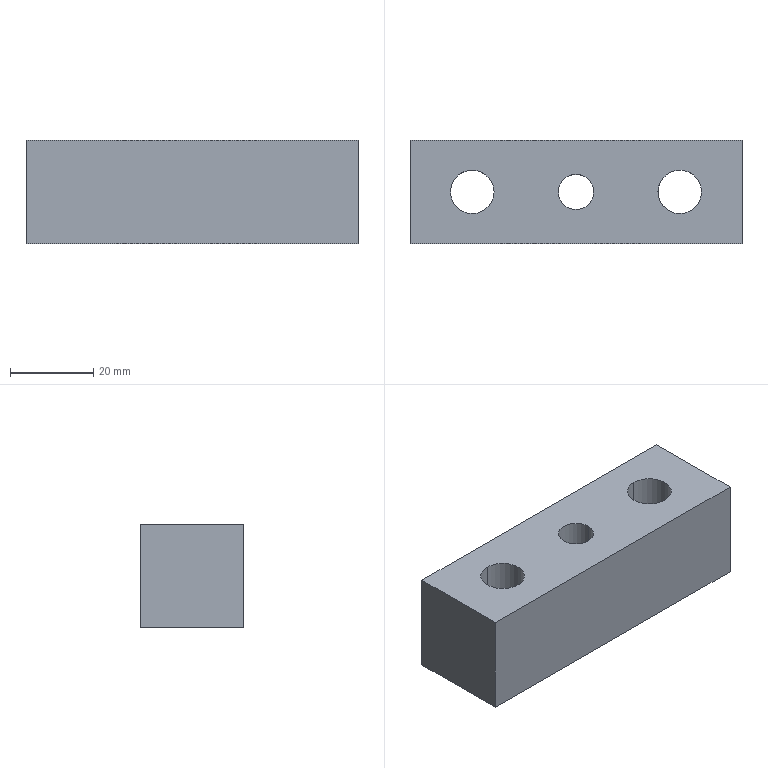Part | STEP file | 1_id1602_x_t | 1 solid | 18 faces | box 80 x 25 x 25 mm | volume 40040 mm3 | cylinder 10 | plane 8 | commonest cylinder face diameters 10.5 x4 17 x4 8.5 x2
STEP:
#1=CARTESIAN_POINT('',(0.,0.,0.));
#2=DIRECTION('',(0.,0.,1.));
#3=DIRECTION('',(1.,0.,0.));
#4=AXIS2_PLACEMENT_3D('',#1,#2,#3);
#5=CARTESIAN_POINT('',(605.45,-32.376,-77.49));
#6=VERTEX_POINT('',#5);
#7=CARTESIAN_POINT('',(613.95,-32.376,-77.49));
#8=VERTEX_POINT('',#7);
#9=CARTESIAN_POINT('',(609.7,-32.376,-77.49));
#10=DIRECTION('',(0.,0.,-1.));
#11=DIRECTION('',(-1.,0.,0.));
#12=AXIS2_PLACEMENT_3D('',#9,#10,#11);
#13=CIRCLE('',#12,4.25);
#14=CARTESIAN_POINT('',(609.7,-32.376,-73.24));
#15=DIRECTION('',(0.,0.,1.));
#16=DIRECTION('',(-1.,0.,0.));
#17=AXIS2_PLACEMENT_3D('',#14,#15,#16);
#18=CYLINDRICAL_SURFACE('',#17,4.25);
#19=CARTESIAN_POINT('',(6.283,-4.25));
#20=DIRECTION('',(-1.,0.));
#21=VECTOR('',#20,1.);
#22=LINE('',#19,#21);
#23=(GEOMETRIC_REPRESENTATION_CONTEXT(2)PARAMETRIC_REPRESENTATION_CONTEXT()REPRESENTATION_CONTEXT('',''));
#24=DEFINITIONAL_REPRESENTATION('',(#22),#23);
#25=PCURVE('',#18,#24);
#26=CARTESIAN_POINT('',(649.7,-44.876,-77.49));
#27=DIRECTION('',(0.,0.,-1.));
#28=DIRECTION('',(1.,0.,0.));
#29=AXIS2_PLACEMENT_3D('',#26,#27,#28);
#30=PLANE('',#29);
#31=CARTESIAN_POINT('',(-40.,-12.5));
#32=DIRECTION('',(-1.,0.));
#33=AXIS2_PLACEMENT_2D('',#31,#32);
#34=CIRCLE('',#33,4.25);
#35=(GEOMETRIC_REPRESENTATION_CONTEXT(2)PARAMETRIC_REPRESENTATION_CONTEXT()REPRESENTATION_CONTEXT('',''));
#36=DEFINITIONAL_REPRESENTATION('',(#34),#35);
#37=PCURVE('',#30,#36);
#38=SURFACE_CURVE('',#13,(#25,#37),.PCURVE_S1.);
#39=EDGE_CURVE('',#6,#8,#38,.T.);
#40=ORIENTED_EDGE('',*,*,#39,.T.);
#41=CARTESIAN_POINT('',(613.95,-32.376,-102.49));
#42=VERTEX_POINT('',#41);
#43=CARTESIAN_POINT('',(613.95,-32.376,-102.49));
#44=DIRECTION('',(0.,0.,1.));
#45=VECTOR('',#44,1.);
#46=LINE('',#43,#45);
#47=CARTESIAN_POINT('',(3.142,-29.25));
#48=DIRECTION('',(0.,1.));
#49=VECTOR('',#48,1.);
#50=LINE('',#47,#49);
#51=(GEOMETRIC_REPRESENTATION_CONTEXT(2)PARAMETRIC_REPRESENTATION_CONTEXT()REPRESENTATION_CONTEXT('',''));
#52=DEFINITIONAL_REPRESENTATION('',(#50),#51);
#53=PCURVE('',#18,#52);
#54=CARTESIAN_POINT('',(609.7,-32.376,-73.24));
#55=DIRECTION('',(0.,0.,1.));
#56=DIRECTION('',(-1.,0.,0.));
#57=AXIS2_PLACEMENT_3D('',#54,#55,#56);
#58=CYLINDRICAL_SURFACE('',#57,4.25);
#59=CARTESIAN_POINT('',(3.142,-29.25));
#60=DIRECTION('',(0.,1.));
#61=VECTOR('',#60,1.);
#62=LINE('',#59,#61);
#63=(GEOMETRIC_REPRESENTATION_CONTEXT(2)PARAMETRIC_REPRESENTATION_CONTEXT()REPRESENTATION_CONTEXT('',''));
#64=DEFINITIONAL_REPRESENTATION('',(#62),#63);
#65=PCURVE('',#58,#64);
#66=SURFACE_CURVE('',#46,(#53,#65),.PCURVE_S1.);
#67=EDGE_CURVE('',#42,#8,#66,.T.);
#68=ORIENTED_EDGE('',*,*,#67,.F.);
#69=CARTESIAN_POINT('',(605.45,-32.376,-102.49));
#70=VERTEX_POINT('',#69);
#71=CARTESIAN_POINT('',(609.7,-32.376,-102.49));
#72=DIRECTION('',(0.,0.,1.));
#73=DIRECTION('',(1.,0.,0.));
#74=AXIS2_PLACEMENT_3D('',#71,#72,#73);
#75=CIRCLE('',#74,4.25);
#76=CARTESIAN_POINT('',(3.142,-29.25));
#77=DIRECTION('',(1.,0.));
#78=VECTOR('',#77,1.);
#79=LINE('',#76,#78);
#80=(GEOMETRIC_REPRESENTATION_CONTEXT(2)PARAMETRIC_REPRESENTATION_CONTEXT()REPRESENTATION_CONTEXT('',''));
#81=DEFINITIONAL_REPRESENTATION('',(#79),#80);
#82=PCURVE('',#18,#81);
#83=CARTESIAN_POINT('',(649.7,-44.876,-102.49));
#84=DIRECTION('',(0.,0.,-1.));
#85=DIRECTION('',(1.,0.,0.));
#86=AXIS2_PLACEMENT_3D('',#83,#84,#85);
#87=PLANE('',#86);
#88=CARTESIAN_POINT('',(-35.75,-12.5));
#89=CARTESIAN_POINT('',(-35.75,-19.861));
#90=CARTESIAN_POINT('',(-42.125,-16.181));
#91=CARTESIAN_POINT('',(-48.5,-12.5));
#92=CARTESIAN_POINT('',(-42.125,-8.819));
#93=CARTESIAN_POINT('',(-35.75,-5.139));
#94=CARTESIAN_POINT('',(-35.75,-12.5));
#95=(BOUNDED_CURVE()B_SPLINE_CURVE(2,(#88,#89,#90,#91,#92,#93,#94),.UNSPECIFIED.,.T.,.F.)B_SPLINE_CURVE_WITH_KNOTS((1,2,2,2,2,1),(-2.094,0.,2.094,4.189,6.283,8.378),.UNSPECIFIED.)CURVE()GEOMETRIC_REPRESENTATION_ITEM()RATIONAL_B_SPLINE_CURVE((1.,0.5,1.,0.5,1.,0.5,1.))REPRESENTATION_ITEM(''));
#96=(GEOMETRIC_REPRESENTATION_CONTEXT(2)PARAMETRIC_REPRESENTATION_CONTEXT()REPRESENTATION_CONTEXT('',''));
#97=DEFINITIONAL_REPRESENTATION('',(#95),#96);
#98=PCURVE('',#87,#97);
#99=SURFACE_CURVE('',#75,(#82,#98),.PCURVE_S1.);
#100=EDGE_CURVE('',#42,#70,#99,.T.);
#101=ORIENTED_EDGE('',*,*,#100,.T.);
#102=CARTESIAN_POINT('',(605.45,-32.376,-102.49));
#103=DIRECTION('',(0.,0.,-1.));
#104=VECTOR('',#103,1.);
#105=LINE('',#102,#104);
#106=CARTESIAN_POINT('',(6.283,-29.25));
#107=DIRECTION('',(0.,-1.));
#108=VECTOR('',#107,1.);
#109=LINE('',#106,#108);
#110=(GEOMETRIC_REPRESENTATION_CONTEXT(2)PARAMETRIC_REPRESENTATION_CONTEXT()REPRESENTATION_CONTEXT('',''));
#111=DEFINITIONAL_REPRESENTATION('',(#109),#110);
#112=PCURVE('',#18,#111);
#113=CARTESIAN_POINT('',(0.,-29.25));
#114=DIRECTION('',(0.,-1.));
#115=VECTOR('',#114,1.);
#116=LINE('',#113,#115);
#117=(GEOMETRIC_REPRESENTATION_CONTEXT(2)PARAMETRIC_REPRESENTATION_CONTEXT()REPRESENTATION_CONTEXT('',''));
#118=DEFINITIONAL_REPRESENTATION('',(#116),#117);
#119=PCURVE('',#58,#118);
#120=SURFACE_CURVE('',#105,(#112,#119),.PCURVE_S1.);
#121=EDGE_CURVE('',#6,#70,#120,.T.);
#122=ORIENTED_EDGE('',*,*,#121,.F.);
#123=EDGE_LOOP('',(#40,#68,#101,#122));
#124=FACE_BOUND('',#123,.F.);
#125=ADVANCED_FACE('',(#124),#18,.F.);
#126=CARTESIAN_POINT('',(649.7,-19.876,-77.49));
#127=VERTEX_POINT('',#126);
#128=CARTESIAN_POINT('',(569.7,-19.876,-77.49));
#129=VERTEX_POINT('',#128);
#130=CARTESIAN_POINT('',(649.7,-19.876,-77.49));
#131=DIRECTION('',(-1.,0.,0.));
#132=VECTOR('',#131,1.);
#133=LINE('',#130,#132);
#134=CARTESIAN_POINT('',(0.,-25.));
#135=DIRECTION('',(-1.,0.));
#136=VECTOR('',#135,1.);
#137=LINE('',#134,#136);
#138=(GEOMETRIC_REPRESENTATION_CONTEXT(2)PARAMETRIC_REPRESENTATION_CONTEXT()REPRESENTATION_CONTEXT('',''));
#139=DEFINITIONAL_REPRESENTATION('',(#137),#138);
#140=PCURVE('',#30,#139);
#141=CARTESIAN_POINT('',(569.7,-19.876,-77.49));
#142=DIRECTION('',(0.,1.,0.));
#143=DIRECTION('',(1.,0.,0.));
#144=AXIS2_PLACEMENT_3D('',#141,#142,#143);
#145=PLANE('',#144);
#146=CARTESIAN_POINT('',(80.,0.));
#147=DIRECTION('',(-1.,0.));
#148=VECTOR('',#147,1.);
#149=LINE('',#146,#148);
#150=(GEOMETRIC_REPRESENTATION_CONTEXT(2)PARAMETRIC_REPRESENTATION_CONTEXT()REPRESENTATION_CONTEXT('',''));
#151=DEFINITIONAL_REPRESENTATION('',(#149),#150);
#152=PCURVE('',#145,#151);
#153=SURFACE_CURVE('',#133,(#140,#152),.PCURVE_S1.);
#154=EDGE_CURVE('',#127,#129,#153,.T.);
#155=ORIENTED_EDGE('',*,*,#154,.T.);
#156=CARTESIAN_POINT('',(569.7,-44.876,-77.49));
#157=VERTEX_POINT('',#156);
#158=CARTESIAN_POINT('',(569.7,-19.876,-77.49));
#159=DIRECTION('',(0.,-1.,0.));
#160=VECTOR('',#159,1.);
#161=LINE('',#158,#160);
#162=CARTESIAN_POINT('',(-80.,-25.));
#163=DIRECTION('',(0.,1.));
#164=VECTOR('',#163,1.);
#165=LINE('',#162,#164);
#166=(GEOMETRIC_REPRESENTATION_CONTEXT(2)PARAMETRIC_REPRESENTATION_CONTEXT()REPRESENTATION_CONTEXT('',''));
#167=DEFINITIONAL_REPRESENTATION('',(#165),#166);
#168=PCURVE('',#30,#167);
#169=CARTESIAN_POINT('',(569.7,-44.876,-77.49));
#170=DIRECTION('',(-1.,0.,0.));
#171=DIRECTION('',(0.,-1.,0.));
#172=AXIS2_PLACEMENT_3D('',#169,#170,#171);
#173=PLANE('',#172);
#174=CARTESIAN_POINT('',(-25.,0.));
#175=DIRECTION('',(1.,0.));
#176=VECTOR('',#175,1.);
#177=LINE('',#174,#176);
#178=(GEOMETRIC_REPRESENTATION_CONTEXT(2)PARAMETRIC_REPRESENTATION_CONTEXT()REPRESENTATION_CONTEXT('',''));
#179=DEFINITIONAL_REPRESENTATION('',(#177),#178);
#180=PCURVE('',#173,#179);
#181=SURFACE_CURVE('',#161,(#168,#180),.PCURVE_S1.);
#182=EDGE_CURVE('',#129,#157,#181,.T.);
#183=ORIENTED_EDGE('',*,*,#182,.T.);
#184=CARTESIAN_POINT('',(649.7,-44.876,-77.49));
#185=VERTEX_POINT('',#184);
#186=CARTESIAN_POINT('',(569.7,-44.876,-77.49));
#187=DIRECTION('',(1.,0.,0.));
#188=VECTOR('',#187,1.);
#189=LINE('',#186,#188);
#190=CARTESIAN_POINT('',(-80.,0.));
#191=DIRECTION('',(1.,0.));
#192=VECTOR('',#191,1.);
#193=LINE('',#190,#192);
#194=(GEOMETRIC_REPRESENTATION_CONTEXT(2)PARAMETRIC_REPRESENTATION_CONTEXT()REPRESENTATION_CONTEXT('',''));
#195=DEFINITIONAL_REPRESENTATION('',(#193),#194);
#196=PCURVE('',#30,#195);
#197=CARTESIAN_POINT('',(649.7,-44.876,-77.49));
#198=DIRECTION('',(0.,-1.,0.));
#199=DIRECTION('',(0.,0.,-1.));
#200=AXIS2_PLACEMENT_3D('',#197,#198,#199);
#201=PLANE('',#200);
#202=CARTESIAN_POINT('',(0.,-80.));
#203=DIRECTION('',(0.,1.));
#204=VECTOR('',#203,1.);
#205=LINE('',#202,#204);
#206=(GEOMETRIC_REPRESENTATION_CONTEXT(2)PARAMETRIC_REPRESENTATION_CONTEXT()REPRESENTATION_CONTEXT('',''));
#207=DEFINITIONAL_REPRESENTATION('',(#205),#206);
#208=PCURVE('',#201,#207);
#209=SURFACE_CURVE('',#189,(#196,#208),.PCURVE_S1.);
#210=EDGE_CURVE('',#157,#185,#209,.T.);
#211=ORIENTED_EDGE('',*,*,#210,.T.);
#212=CARTESIAN_POINT('',(649.7,-44.876,-77.49));
#213=DIRECTION('',(0.,1.,0.));
#214=VECTOR('',#213,1.);
#215=LINE('',#212,#214);
#216=CARTESIAN_POINT('',(0.,0.));
#217=DIRECTION('',(0.,-1.));
#218=VECTOR('',#217,1.);
#219=LINE('',#216,#218);
#220=(GEOMETRIC_REPRESENTATION_CONTEXT(2)PARAMETRIC_REPRESENTATION_CONTEXT()REPRESENTATION_CONTEXT('',''));
#221=DEFINITIONAL_REPRESENTATION('',(#219),#220);
#222=PCURVE('',#30,#221);
#223=CARTESIAN_POINT('',(649.7,-19.876,-77.49));
#224=DIRECTION('',(1.,0.,0.));
#225=DIRECTION('',(0.,0.,1.));
#226=AXIS2_PLACEMENT_3D('',#223,#224,#225);
#227=PLANE('',#226);
#228=CARTESIAN_POINT('',(0.,25.));
#229=DIRECTION('',(0.,-1.));
#230=VECTOR('',#229,1.);
#231=LINE('',#228,#230);
#232=(GEOMETRIC_REPRESENTATION_CONTEXT(2)PARAMETRIC_REPRESENTATION_CONTEXT()REPRESENTATION_CONTEXT('',''));
#233=DEFINITIONAL_REPRESENTATION('',(#231),#232);
#234=PCURVE('',#227,#233);
#235=SURFACE_CURVE('',#215,(#222,#234),.PCURVE_S1.);
#236=EDGE_CURVE('',#185,#127,#235,.T.);
#237=ORIENTED_EDGE('',*,*,#236,.T.);
#238=EDGE_LOOP('',(#155,#183,#211,#237));
#239=FACE_BOUND('',#238,.T.);
#240=CARTESIAN_POINT('',(634.7,-27.126,-77.49));
#241=VERTEX_POINT('',#240);
#242=CARTESIAN_POINT('',(639.95,-32.376,-77.49));
#243=VERTEX_POINT('',#242);
#244=CARTESIAN_POINT('',(634.7,-32.376,-77.49));
#245=DIRECTION('',(0.,0.,-1.));
#246=DIRECTION('',(0.,1.,0.));
#247=AXIS2_PLACEMENT_3D('',#244,#245,#246);
#248=CIRCLE('',#247,5.25);
#249=CARTESIAN_POINT('',(-15.,-12.5));
#250=DIRECTION('',(0.,-1.));
#251=AXIS2_PLACEMENT_2D('',#249,#250);
#252=CIRCLE('',#251,5.25);
#253=(GEOMETRIC_REPRESENTATION_CONTEXT(2)PARAMETRIC_REPRESENTATION_CONTEXT()REPRESENTATION_CONTEXT('',''));
#254=DEFINITIONAL_REPRESENTATION('',(#252),#253);
#255=PCURVE('',#30,#254);
#256=CARTESIAN_POINT('',(634.7,-32.376,-77.24));
#257=DIRECTION('',(0.,0.,1.));
#258=DIRECTION('',(0.,-1.,0.));
#259=AXIS2_PLACEMENT_3D('',#256,#257,#258);
#260=CYLINDRICAL_SURFACE('',#259,5.25);
#261=CARTESIAN_POINT('',(3.142,-0.25));
#262=DIRECTION('',(-1.,0.));
#263=VECTOR('',#262,1.);
#264=LINE('',#261,#263);
#265=(GEOMETRIC_REPRESENTATION_CONTEXT(2)PARAMETRIC_REPRESENTATION_CONTEXT()REPRESENTATION_CONTEXT('',''));
#266=DEFINITIONAL_REPRESENTATION('',(#264),#265);
#267=PCURVE('',#260,#266);
#268=SURFACE_CURVE('',#248,(#255,#267),.PCURVE_S1.);
#269=EDGE_CURVE('',#241,#243,#268,.T.);
#270=ORIENTED_EDGE('',*,*,#269,.T.);
#271=CARTESIAN_POINT('',(634.7,-37.626,-77.49));
#272=VERTEX_POINT('',#271);
#273=CARTESIAN_POINT('',(634.7,-32.376,-77.49));
#274=DIRECTION('',(0.,0.,-1.));
#275=DIRECTION('',(1.,0.,0.));
#276=AXIS2_PLACEMENT_3D('',#273,#274,#275);
#277=CIRCLE('',#276,5.25);
#278=CARTESIAN_POINT('',(-15.,-12.5));
#279=DIRECTION('',(1.,0.));
#280=AXIS2_PLACEMENT_2D('',#278,#279);
#281=CIRCLE('',#280,5.25);
#282=(GEOMETRIC_REPRESENTATION_CONTEXT(2)PARAMETRIC_REPRESENTATION_CONTEXT()REPRESENTATION_CONTEXT('',''));
#283=DEFINITIONAL_REPRESENTATION('',(#281),#282);
#284=PCURVE('',#30,#283);
#285=CARTESIAN_POINT('',(1.571,-0.25));
#286=DIRECTION('',(-1.,0.));
#287=VECTOR('',#286,1.);
#288=LINE('',#285,#287);
#289=(GEOMETRIC_REPRESENTATION_CONTEXT(2)PARAMETRIC_REPRESENTATION_CONTEXT()REPRESENTATION_CONTEXT('',''));
#290=DEFINITIONAL_REPRESENTATION('',(#288),#289);
#291=PCURVE('',#260,#290);
#292=SURFACE_CURVE('',#277,(#284,#291),.PCURVE_S1.);
#293=EDGE_CURVE('',#243,#272,#292,.T.);
#294=ORIENTED_EDGE('',*,*,#293,.T.);
#295=CARTESIAN_POINT('',(629.45,-32.376,-77.49));
#296=VERTEX_POINT('',#295);
#297=CARTESIAN_POINT('',(634.7,-32.376,-77.49));
#298=DIRECTION('',(0.,0.,-1.));
#299=DIRECTION('',(0.,-1.,0.));
#300=AXIS2_PLACEMENT_3D('',#297,#298,#299);
#301=CIRCLE('',#300,5.25);
#302=CARTESIAN_POINT('',(-15.,-12.5));
#303=DIRECTION('',(0.,1.));
#304=AXIS2_PLACEMENT_2D('',#302,#303);
#305=CIRCLE('',#304,5.25);
#306=(GEOMETRIC_REPRESENTATION_CONTEXT(2)PARAMETRIC_REPRESENTATION_CONTEXT()REPRESENTATION_CONTEXT('',''));
#307=DEFINITIONAL_REPRESENTATION('',(#305),#306);
#308=PCURVE('',#30,#307);
#309=CARTESIAN_POINT('',(634.7,-32.376,-77.24));
#310=DIRECTION('',(0.,0.,1.));
#311=DIRECTION('',(0.,-1.,0.));
#312=AXIS2_PLACEMENT_3D('',#309,#310,#311);
#313=CYLINDRICAL_SURFACE('',#312,5.25);
#314=CARTESIAN_POINT('',(6.283,-0.25));
#315=DIRECTION('',(-1.,0.));
#316=VECTOR('',#315,1.);
#317=LINE('',#314,#316);
#318=(GEOMETRIC_REPRESENTATION_CONTEXT(2)PARAMETRIC_REPRESENTATION_CONTEXT()REPRESENTATION_CONTEXT('',''));
#319=DEFINITIONAL_REPRESENTATION('',(#317),#318);
#320=PCURVE('',#313,#319);
#321=SURFACE_CURVE('',#301,(#308,#320),.PCURVE_S1.);
#322=EDGE_CURVE('',#272,#296,#321,.T.);
#323=ORIENTED_EDGE('',*,*,#322,.T.);
#324=CARTESIAN_POINT('',(634.7,-32.376,-77.49));
#325=DIRECTION('',(0.,0.,-1.));
#326=DIRECTION('',(-1.,0.,0.));
#327=AXIS2_PLACEMENT_3D('',#324,#325,#326);
#328=CIRCLE('',#327,5.25);
#329=CARTESIAN_POINT('',(-15.,-12.5));
#330=DIRECTION('',(-1.,0.));
#331=AXIS2_PLACEMENT_2D('',#329,#330);
#332=CIRCLE('',#331,5.25);
#333=(GEOMETRIC_REPRESENTATION_CONTEXT(2)PARAMETRIC_REPRESENTATION_CONTEXT()REPRESENTATION_CONTEXT('',''));
#334=DEFINITIONAL_REPRESENTATION('',(#332),#333);
#335=PCURVE('',#30,#334);
#336=CARTESIAN_POINT('',(4.712,-0.25));
#337=DIRECTION('',(-1.,0.));
#338=VECTOR('',#337,1.);
#339=LINE('',#336,#338);
#340=(GEOMETRIC_REPRESENTATION_CONTEXT(2)PARAMETRIC_REPRESENTATION_CONTEXT()REPRESENTATION_CONTEXT('',''));
#341=DEFINITIONAL_REPRESENTATION('',(#339),#340);
#342=PCURVE('',#313,#341);
#343=SURFACE_CURVE('',#328,(#335,#342),.PCURVE_S1.);
#344=EDGE_CURVE('',#296,#241,#343,.T.);
#345=ORIENTED_EDGE('',*,*,#344,.T.);
#346=EDGE_LOOP('',(#270,#294,#323,#345));
#347=FACE_BOUND('',#346,.T.);
#348=CARTESIAN_POINT('',(609.7,-32.376,-77.49));
#349=DIRECTION('',(0.,0.,-1.));
#350=DIRECTION('',(1.,0.,0.));
#351=AXIS2_PLACEMENT_3D('',#348,#349,#350);
#352=CIRCLE('',#351,4.25);
#353=CARTESIAN_POINT('',(-40.,-12.5));
#354=DIRECTION('',(1.,0.));
#355=AXIS2_PLACEMENT_2D('',#353,#354);
#356=CIRCLE('',#355,4.25);
#357=(GEOMETRIC_REPRESENTATION_CONTEXT(2)PARAMETRIC_REPRESENTATION_CONTEXT()REPRESENTATION_CONTEXT('',''));
#358=DEFINITIONAL_REPRESENTATION('',(#356),#357);
#359=PCURVE('',#30,#358);
#360=CARTESIAN_POINT('',(3.142,-4.25));
#361=DIRECTION('',(-1.,0.));
#362=VECTOR('',#361,1.);
#363=LINE('',#360,#362);
#364=(GEOMETRIC_REPRESENTATION_CONTEXT(2)PARAMETRIC_REPRESENTATION_CONTEXT()REPRESENTATION_CONTEXT('',''));
#365=DEFINITIONAL_REPRESENTATION('',(#363),#364);
#366=PCURVE('',#58,#365);
#367=SURFACE_CURVE('',#352,(#359,#366),.PCURVE_S1.);
#368=EDGE_CURVE('',#8,#6,#367,.T.);
#369=ORIENTED_EDGE('',*,*,#368,.T.);
#370=ORIENTED_EDGE('',*,*,#39,.T.);
#371=EDGE_LOOP('',(#369,#370));
#372=FACE_BOUND('',#371,.T.);
#373=CARTESIAN_POINT('',(584.7,-27.126,-77.49));
#374=VERTEX_POINT('',#373);
#375=CARTESIAN_POINT('',(589.95,-32.376,-77.49));
#376=VERTEX_POINT('',#375);
#377=CARTESIAN_POINT('',(584.7,-32.376,-77.49));
#378=DIRECTION('',(0.,0.,-1.));
#379=DIRECTION('',(0.,1.,0.));
#380=AXIS2_PLACEMENT_3D('',#377,#378,#379);
#381=CIRCLE('',#380,5.25);
#382=CARTESIAN_POINT('',(-65.,-12.5));
#383=DIRECTION('',(0.,-1.));
#384=AXIS2_PLACEMENT_2D('',#382,#383);
#385=CIRCLE('',#384,5.25);
#386=(GEOMETRIC_REPRESENTATION_CONTEXT(2)PARAMETRIC_REPRESENTATION_CONTEXT()REPRESENTATION_CONTEXT('',''));
#387=DEFINITIONAL_REPRESENTATION('',(#385),#386);
#388=PCURVE('',#30,#387);
#389=CARTESIAN_POINT('',(584.7,-32.376,-77.24));
#390=DIRECTION('',(0.,0.,1.));
#391=DIRECTION('',(0.,-1.,0.));
#392=AXIS2_PLACEMENT_3D('',#389,#390,#391);
#393=CYLINDRICAL_SURFACE('',#392,5.25);
#394=CARTESIAN_POINT('',(3.142,-0.25));
#395=DIRECTION('',(-1.,0.));
#396=VECTOR('',#395,1.);
#397=LINE('',#394,#396);
#398=(GEOMETRIC_REPRESENTATION_CONTEXT(2)PARAMETRIC_REPRESENTATION_CONTEXT()REPRESENTATION_CONTEXT('',''));
#399=DEFINITIONAL_REPRESENTATION('',(#397),#398);
#400=PCURVE('',#393,#399);
#401=SURFACE_CURVE('',#381,(#388,#400),.PCURVE_S1.);
#402=EDGE_CURVE('',#374,#376,#401,.T.);
#403=ORIENTED_EDGE('',*,*,#402,.T.);
#404=CARTESIAN_POINT('',(584.7,-37.626,-77.49));
#405=VERTEX_POINT('',#404);
#406=CARTESIAN_POINT('',(584.7,-32.376,-77.49));
#407=DIRECTION('',(0.,0.,-1.));
#408=DIRECTION('',(1.,0.,0.));
#409=AXIS2_PLACEMENT_3D('',#406,#407,#408);
#410=CIRCLE('',#409,5.25);
#411=CARTESIAN_POINT('',(-65.,-12.5));
#412=DIRECTION('',(1.,0.));
#413=AXIS2_PLACEMENT_2D('',#411,#412);
#414=CIRCLE('',#413,5.25);
#415=(GEOMETRIC_REPRESENTATION_CONTEXT(2)PARAMETRIC_REPRESENTATION_CONTEXT()REPRESENTATION_CONTEXT('',''));
#416=DEFINITIONAL_REPRESENTATION('',(#414),#415);
#417=PCURVE('',#30,#416);
#418=CARTESIAN_POINT('',(1.571,-0.25));
#419=DIRECTION('',(-1.,0.));
#420=VECTOR('',#419,1.);
#421=LINE('',#418,#420);
#422=(GEOMETRIC_REPRESENTATION_CONTEXT(2)PARAMETRIC_REPRESENTATION_CONTEXT()REPRESENTATION_CONTEXT('',''));
#423=DEFINITIONAL_REPRESENTATION('',(#421),#422);
#424=PCURVE('',#393,#423);
#425=SURFACE_CURVE('',#410,(#417,#424),.PCURVE_S1.);
#426=EDGE_CURVE('',#376,#405,#425,.T.);
#427=ORIENTED_EDGE('',*,*,#426,.T.);
#428=CARTESIAN_POINT('',(579.45,-32.376,-77.49));
#429=VERTEX_POINT('',#428);
#430=CARTESIAN_POINT('',(584.7,-32.376,-77.49));
#431=DIRECTION('',(0.,0.,-1.));
#432=DIRECTION('',(0.,-1.,0.));
#433=AXIS2_PLACEMENT_3D('',#430,#431,#432);
#434=CIRCLE('',#433,5.25);
#435=CARTESIAN_POINT('',(-65.,-12.5));
#436=DIRECTION('',(0.,1.));
#437=AXIS2_PLACEMENT_2D('',#435,#436);
#438=CIRCLE('',#437,5.25);
#439=(GEOMETRIC_REPRESENTATION_CONTEXT(2)PARAMETRIC_REPRESENTATION_CONTEXT()REPRESENTATION_CONTEXT('',''));
#440=DEFINITIONAL_REPRESENTATION('',(#438),#439);
#441=PCURVE('',#30,#440);
#442=CARTESIAN_POINT('',(584.7,-32.376,-77.24));
#443=DIRECTION('',(0.,0.,1.));
#444=DIRECTION('',(0.,-1.,0.));
#445=AXIS2_PLACEMENT_3D('',#442,#443,#444);
#446=CYLINDRICAL_SURFACE('',#445,5.25);
#447=CARTESIAN_POINT('',(6.283,-0.25));
#448=DIRECTION('',(-1.,0.));
#449=VECTOR('',#448,1.);
#450=LINE('',#447,#449);
#451=(GEOMETRIC_REPRESENTATION_CONTEXT(2)PARAMETRIC_REPRESENTATION_CONTEXT()REPRESENTATION_CONTEXT('',''));
#452=DEFINITIONAL_REPRESENTATION('',(#450),#451);
#453=PCURVE('',#446,#452);
#454=SURFACE_CURVE('',#434,(#441,#453),.PCURVE_S1.);
#455=EDGE_CURVE('',#405,#429,#454,.T.);
#456=ORIENTED_EDGE('',*,*,#455,.T.);
#457=CARTESIAN_POINT('',(584.7,-32.376,-77.49));
#458=DIRECTION('',(0.,0.,-1.));
#459=DIRECTION('',(-1.,0.,0.));
#460=AXIS2_PLACEMENT_3D('',#457,#458,#459);
#461=CIRCLE('',#460,5.25);
#462=CARTESIAN_POINT('',(-65.,-12.5));
#463=DIRECTION('',(-1.,0.));
#464=AXIS2_PLACEMENT_2D('',#462,#463);
#465=CIRCLE('',#464,5.25);
#466=(GEOMETRIC_REPRESENTATION_CONTEXT(2)PARAMETRIC_REPRESENTATION_CONTEXT()REPRESENTATION_CONTEXT('',''));
#467=DEFINITIONAL_REPRESENTATION('',(#465),#466);
#468=PCURVE('',#30,#467);
#469=CARTESIAN_POINT('',(4.712,-0.25));
#470=DIRECTION('',(-1.,0.));
#471=VECTOR('',#470,1.);
#472=LINE('',#469,#471);
#473=(GEOMETRIC_REPRESENTATION_CONTEXT(2)PARAMETRIC_REPRESENTATION_CONTEXT()REPRESENTATION_CONTEXT('',''));
#474=DEFINITIONAL_REPRESENTATION('',(#472),#473);
#475=PCURVE('',#446,#474);
#476=SURFACE_CURVE('',#461,(#468,#475),.PCURVE_S1.);
#477=EDGE_CURVE('',#429,#374,#476,.T.);
#478=ORIENTED_EDGE('',*,*,#477,.T.);
#479=EDGE_LOOP('',(#403,#427,#456,#478));
#480=FACE_BOUND('',#479,.T.);
#481=ADVANCED_FACE('',(#239,#347,#372,#480),#30,.F.);
#482=ORIENTED_EDGE('',*,*,#322,.T.);
#483=ORIENTED_EDGE('',*,*,#344,.T.);
#484=CARTESIAN_POINT('',(634.7,-27.126,-87.49));
#485=VERTEX_POINT('',#484);
#486=CARTESIAN_POINT('',(634.7,-27.126,-87.49));
#487=DIRECTION('',(0.,0.,1.));
#488=VECTOR('',#487,1.);
#489=LINE('',#486,#488);
#490=CARTESIAN_POINT('',(3.142,-10.25));
#491=DIRECTION('',(0.,1.));
#492=VECTOR('',#491,1.);
#493=LINE('',#490,#492);
#494=(GEOMETRIC_REPRESENTATION_CONTEXT(2)PARAMETRIC_REPRESENTATION_CONTEXT()REPRESENTATION_CONTEXT('',''));
#495=DEFINITIONAL_REPRESENTATION('',(#493),#494);
#496=PCURVE('',#313,#495);
#497=CARTESIAN_POINT('',(3.142,-10.25));
#498=DIRECTION('',(0.,1.));
#499=VECTOR('',#498,1.);
#500=LINE('',#497,#499);
#501=(GEOMETRIC_REPRESENTATION_CONTEXT(2)PARAMETRIC_REPRESENTATION_CONTEXT()REPRESENTATION_CONTEXT('',''));
#502=DEFINITIONAL_REPRESENTATION('',(#500),#501);
#503=PCURVE('',#260,#502);
#504=SURFACE_CURVE('',#489,(#496,#503),.PCURVE_S1.);
#505=EDGE_CURVE('',#485,#241,#504,.T.);
#506=ORIENTED_EDGE('',*,*,#505,.F.);
#507=CARTESIAN_POINT('',(634.7,-37.626,-87.49));
#508=VERTEX_POINT('',#507);
#509=CARTESIAN_POINT('',(634.7,-32.376,-87.49));
#510=DIRECTION('',(0.,0.,1.));
#511=DIRECTION('',(0.,1.,0.));
#512=AXIS2_PLACEMENT_3D('',#509,#510,#511);
#513=CIRCLE('',#512,5.25);
#514=CARTESIAN_POINT('',(3.142,-10.25));
#515=DIRECTION('',(1.,0.));
#516=VECTOR('',#515,1.);
#517=LINE('',#514,#516);
#518=(GEOMETRIC_REPRESENTATION_CONTEXT(2)PARAMETRIC_REPRESENTATION_CONTEXT()REPRESENTATION_CONTEXT('',''));
#519=DEFINITIONAL_REPRESENTATION('',(#517),#518);
#520=PCURVE('',#313,#519);
#521=CARTESIAN_POINT('',(634.7,-32.376,-87.49));
#522=DIRECTION('',(0.,0.,1.));
#523=DIRECTION('',(0.,1.,0.));
#524=AXIS2_PLACEMENT_3D('',#521,#522,#523);
#525=PLANE('',#524);
#526=CARTESIAN_POINT('',(0.,0.));
#527=DIRECTION('',(1.,0.));
#528=AXIS2_PLACEMENT_2D('',#526,#527);
#529=CIRCLE('',#528,5.25);
#530=(GEOMETRIC_REPRESENTATION_CONTEXT(2)PARAMETRIC_REPRESENTATION_CONTEXT()REPRESENTATION_CONTEXT('',''));
#531=DEFINITIONAL_REPRESENTATION('',(#529),#530);
#532=PCURVE('',#525,#531);
#533=SURFACE_CURVE('',#513,(#520,#532),.PCURVE_S1.);
#534=EDGE_CURVE('',#485,#508,#533,.T.);
#535=ORIENTED_EDGE('',*,*,#534,.T.);
#536=CARTESIAN_POINT('',(634.7,-37.626,-87.49));
#537=DIRECTION('',(0.,0.,-1.));
#538=VECTOR('',#537,1.);
#539=LINE('',#536,#538);
#540=CARTESIAN_POINT('',(6.283,-10.25));
#541=DIRECTION('',(0.,-1.));
#542=VECTOR('',#541,1.);
#543=LINE('',#540,#542);
#544=(GEOMETRIC_REPRESENTATION_CONTEXT(2)PARAMETRIC_REPRESENTATION_CONTEXT()REPRESENTATION_CONTEXT('',''));
#545=DEFINITIONAL_REPRESENTATION('',(#543),#544);
#546=PCURVE('',#313,#545);
#547=CARTESIAN_POINT('',(0.,-10.25));
#548=DIRECTION('',(0.,-1.));
#549=VECTOR('',#548,1.);
#550=LINE('',#547,#549);
#551=(GEOMETRIC_REPRESENTATION_CONTEXT(2)PARAMETRIC_REPRESENTATION_CONTEXT()REPRESENTATION_CONTEXT('',''));
#552=DEFINITIONAL_REPRESENTATION('',(#550),#551);
#553=PCURVE('',#260,#552);
#554=SURFACE_CURVE('',#539,(#546,#553),.PCURVE_S1.);
#555=EDGE_CURVE('',#272,#508,#554,.T.);
#556=ORIENTED_EDGE('',*,*,#555,.F.);
#557=EDGE_LOOP('',(#482,#483,#506,#535,#556));
#558=FACE_BOUND('',#557,.F.);
#559=ADVANCED_FACE('',(#558),#313,.F.);
#560=ORIENTED_EDGE('',*,*,#293,.T.);
#561=ORIENTED_EDGE('',*,*,#555,.T.);
#562=CARTESIAN_POINT('',(639.95,-32.376,-87.49));
#563=VERTEX_POINT('',#562);
#564=CARTESIAN_POINT('',(634.7,-32.376,-87.49));
#565=DIRECTION('',(0.,0.,1.));
#566=DIRECTION('',(0.,-1.,0.));
#567=AXIS2_PLACEMENT_3D('',#564,#565,#566);
#568=CIRCLE('',#567,5.25);
#569=CARTESIAN_POINT('',(0.,-10.25));
#570=DIRECTION('',(1.,0.));
#571=VECTOR('',#570,1.);
#572=LINE('',#569,#571);
#573=(GEOMETRIC_REPRESENTATION_CONTEXT(2)PARAMETRIC_REPRESENTATION_CONTEXT()REPRESENTATION_CONTEXT('',''));
#574=DEFINITIONAL_REPRESENTATION('',(#572),#573);
#575=PCURVE('',#260,#574);
#576=CARTESIAN_POINT('',(0.,0.));
#577=DIRECTION('',(-1.,0.));
#578=AXIS2_PLACEMENT_2D('',#576,#577);
#579=CIRCLE('',#578,5.25);
#580=(GEOMETRIC_REPRESENTATION_CONTEXT(2)PARAMETRIC_REPRESENTATION_CONTEXT()REPRESENTATION_CONTEXT('',''));
#581=DEFINITIONAL_REPRESENTATION('',(#579),#580);
#582=PCURVE('',#525,#581);
#583=SURFACE_CURVE('',#568,(#575,#582),.PCURVE_S1.);
#584=EDGE_CURVE('',#508,#563,#583,.T.);
#585=ORIENTED_EDGE('',*,*,#584,.T.);
#586=CARTESIAN_POINT('',(634.7,-32.376,-87.49));
#587=DIRECTION('',(0.,0.,1.));
#588=DIRECTION('',(1.,0.,0.));
#589=AXIS2_PLACEMENT_3D('',#586,#587,#588);
#590=CIRCLE('',#589,5.25);
#591=CARTESIAN_POINT('',(1.571,-10.25));
#592=DIRECTION('',(1.,0.));
#593=VECTOR('',#592,1.);
#594=LINE('',#591,#593);
#595=(GEOMETRIC_REPRESENTATION_CONTEXT(2)PARAMETRIC_REPRESENTATION_CONTEXT()REPRESENTATION_CONTEXT('',''));
#596=DEFINITIONAL_REPRESENTATION('',(#594),#595);
#597=PCURVE('',#260,#596);
#598=CARTESIAN_POINT('',(0.,0.));
#599=DIRECTION('',(0.,-1.));
#600=AXIS2_PLACEMENT_2D('',#598,#599);
#601=CIRCLE('',#600,5.25);
#602=(GEOMETRIC_REPRESENTATION_CONTEXT(2)PARAMETRIC_REPRESENTATION_CONTEXT()REPRESENTATION_CONTEXT('',''));
#603=DEFINITIONAL_REPRESENTATION('',(#601),#602);
#604=PCURVE('',#525,#603);
#605=SURFACE_CURVE('',#590,(#597,#604),.PCURVE_S1.);
#606=EDGE_CURVE('',#563,#485,#605,.T.);
#607=ORIENTED_EDGE('',*,*,#606,.T.);
#608=ORIENTED_EDGE('',*,*,#505,.T.);
#609=ORIENTED_EDGE('',*,*,#269,.T.);
#610=EDGE_LOOP('',(#560,#561,#585,#607,#608,#609));
#611=FACE_BOUND('',#610,.F.);
#612=ADVANCED_FACE('',(#611),#260,.F.);
#613=CARTESIAN_POINT('',(634.7,-40.876,-87.49));
#614=VERTEX_POINT('',#613);
#615=CARTESIAN_POINT('',(634.7,-23.876,-87.49));
#616=VERTEX_POINT('',#615);
#617=CARTESIAN_POINT('',(634.7,-32.376,-87.49));
#618=DIRECTION('',(0.,0.,-1.));
#619=DIRECTION('',(0.,-1.,0.));
#620=AXIS2_PLACEMENT_3D('',#617,#618,#619);
#621=CIRCLE('',#620,8.5);
#622=CARTESIAN_POINT('',(-8.5,0.));
#623=CARTESIAN_POINT('',(-8.5,14.722));
#624=CARTESIAN_POINT('',(4.25,7.361));
#625=CARTESIAN_POINT('',(17.,0.));
#626=CARTESIAN_POINT('',(4.25,-7.361));
#627=CARTESIAN_POINT('',(-8.5,-14.722));
#628=CARTESIAN_POINT('',(-8.5,0.));
#629=(BOUNDED_CURVE()B_SPLINE_CURVE(2,(#622,#623,#624,#625,#626,#627,#628),.UNSPECIFIED.,.T.,.F.)B_SPLINE_CURVE_WITH_KNOTS((1,2,2,2,2,1),(-2.094,0.,2.094,4.189,6.283,8.378),.UNSPECIFIED.)CURVE()GEOMETRIC_REPRESENTATION_ITEM()RATIONAL_B_SPLINE_CURVE((1.,0.5,1.,0.5,1.,0.5,1.))REPRESENTATION_ITEM(''));
#630=(GEOMETRIC_REPRESENTATION_CONTEXT(2)PARAMETRIC_REPRESENTATION_CONTEXT()REPRESENTATION_CONTEXT('',''));
#631=DEFINITIONAL_REPRESENTATION('',(#629),#630);
#632=PCURVE('',#525,#631);
#633=CARTESIAN_POINT('',(634.7,-32.376,-87.49));
#634=DIRECTION('',(0.,0.,1.));
#635=DIRECTION('',(0.,-1.,0.));
#636=AXIS2_PLACEMENT_3D('',#633,#634,#635);
#637=CYLINDRICAL_SURFACE('',#636,8.5);
#638=CARTESIAN_POINT('',(6.283,0.));
#639=DIRECTION('',(-1.,0.));
#640=VECTOR('',#639,1.);
#641=LINE('',#638,#640);
#642=(GEOMETRIC_REPRESENTATION_CONTEXT(2)PARAMETRIC_REPRESENTATION_CONTEXT()REPRESENTATION_CONTEXT('',''));
#643=DEFINITIONAL_REPRESENTATION('',(#641),#642);
#644=PCURVE('',#637,#643);
#645=SURFACE_CURVE('',#621,(#632,#644),.PCURVE_S1.);
#646=EDGE_CURVE('',#614,#616,#645,.T.);
#647=ORIENTED_EDGE('',*,*,#646,.T.);
#648=CARTESIAN_POINT('',(634.7,-32.376,-87.49));
#649=DIRECTION('',(0.,0.,-1.));
#650=DIRECTION('',(0.,1.,0.));
#651=AXIS2_PLACEMENT_3D('',#648,#649,#650);
#652=CIRCLE('',#651,8.5);
#653=CARTESIAN_POINT('',(8.5,0.));
#654=CARTESIAN_POINT('',(8.5,-14.722));
#655=CARTESIAN_POINT('',(-4.25,-7.361));
#656=CARTESIAN_POINT('',(-17.,0.));
#657=CARTESIAN_POINT('',(-4.25,7.361));
#658=CARTESIAN_POINT('',(8.5,14.722));
#659=CARTESIAN_POINT('',(8.5,0.));
#660=(BOUNDED_CURVE()B_SPLINE_CURVE(2,(#653,#654,#655,#656,#657,#658,#659),.UNSPECIFIED.,.T.,.F.)B_SPLINE_CURVE_WITH_KNOTS((1,2,2,2,2,1),(-2.094,0.,2.094,4.189,6.283,8.378),.UNSPECIFIED.)CURVE()GEOMETRIC_REPRESENTATION_ITEM()RATIONAL_B_SPLINE_CURVE((1.,0.5,1.,0.5,1.,0.5,1.))REPRESENTATION_ITEM(''));
#661=(GEOMETRIC_REPRESENTATION_CONTEXT(2)PARAMETRIC_REPRESENTATION_CONTEXT()REPRESENTATION_CONTEXT('',''));
#662=DEFINITIONAL_REPRESENTATION('',(#660),#661);
#663=PCURVE('',#525,#662);
#664=CARTESIAN_POINT('',(634.7,-32.376,-87.49));
#665=DIRECTION('',(0.,0.,1.));
#666=DIRECTION('',(0.,-1.,0.));
#667=AXIS2_PLACEMENT_3D('',#664,#665,#666);
#668=CYLINDRICAL_SURFACE('',#667,8.5);
#669=CARTESIAN_POINT('',(3.142,0.));
#670=DIRECTION('',(-1.,0.));
#671=VECTOR('',#670,1.);
#672=LINE('',#669,#671);
#673=(GEOMETRIC_REPRESENTATION_CONTEXT(2)PARAMETRIC_REPRESENTATION_CONTEXT()REPRESENTATION_CONTEXT('',''));
#674=DEFINITIONAL_REPRESENTATION('',(#672),#673);
#675=PCURVE('',#668,#674);
#676=SURFACE_CURVE('',#652,(#663,#675),.PCURVE_S1.);
#677=EDGE_CURVE('',#616,#614,#676,.T.);
#678=ORIENTED_EDGE('',*,*,#677,.T.);
#679=EDGE_LOOP('',(#647,#678));
#680=FACE_BOUND('',#679,.T.);
#681=ORIENTED_EDGE('',*,*,#534,.T.);
#682=ORIENTED_EDGE('',*,*,#584,.T.);
#683=ORIENTED_EDGE('',*,*,#606,.T.);
#684=EDGE_LOOP('',(#681,#682,#683));
#685=FACE_BOUND('',#684,.T.);
#686=ADVANCED_FACE('',(#680,#685),#525,.F.);
#687=ORIENTED_EDGE('',*,*,#677,.T.);
#688=CARTESIAN_POINT('',(634.7,-40.876,-102.49));
#689=VERTEX_POINT('',#688);
#690=CARTESIAN_POINT('',(634.7,-40.876,-102.49));
#691=DIRECTION('',(0.,0.,1.));
#692=VECTOR('',#691,1.);
#693=LINE('',#690,#692);
#694=CARTESIAN_POINT('',(0.,-15.));
#695=DIRECTION('',(0.,1.));
#696=VECTOR('',#695,1.);
#697=LINE('',#694,#696);
#698=(GEOMETRIC_REPRESENTATION_CONTEXT(2)PARAMETRIC_REPRESENTATION_CONTEXT()REPRESENTATION_CONTEXT('',''));
#699=DEFINITIONAL_REPRESENTATION('',(#697),#698);
#700=PCURVE('',#668,#699);
#701=CARTESIAN_POINT('',(6.283,-15.));
#702=DIRECTION('',(0.,1.));
#703=VECTOR('',#702,1.);
#704=LINE('',#701,#703);
#705=(GEOMETRIC_REPRESENTATION_CONTEXT(2)PARAMETRIC_REPRESENTATION_CONTEXT()REPRESENTATION_CONTEXT('',''));
#706=DEFINITIONAL_REPRESENTATION('',(#704),#705);
#707=PCURVE('',#637,#706);
#708=SURFACE_CURVE('',#693,(#700,#707),.PCURVE_S1.);
#709=EDGE_CURVE('',#689,#614,#708,.T.);
#710=ORIENTED_EDGE('',*,*,#709,.F.);
#711=CARTESIAN_POINT('',(634.7,-23.876,-102.49));
#712=VERTEX_POINT('',#711);
#713=CARTESIAN_POINT('',(634.7,-32.376,-102.49));
#714=DIRECTION('',(0.,0.,1.));
#715=DIRECTION('',(0.,-1.,0.));
#716=AXIS2_PLACEMENT_3D('',#713,#714,#715);
#717=CIRCLE('',#716,8.5);
#718=CARTESIAN_POINT('',(0.,-15.));
#719=DIRECTION('',(1.,0.));
#720=VECTOR('',#719,1.);
#721=LINE('',#718,#720);
#722=(GEOMETRIC_REPRESENTATION_CONTEXT(2)PARAMETRIC_REPRESENTATION_CONTEXT()REPRESENTATION_CONTEXT('',''));
#723=DEFINITIONAL_REPRESENTATION('',(#721),#722);
#724=PCURVE('',#668,#723);
#725=CARTESIAN_POINT('',(-15.,-4.));
#726=CARTESIAN_POINT('',(-0.2776,-4.));
#727=CARTESIAN_POINT('',(-7.639,-16.75));
#728=CARTESIAN_POINT('',(-15.,-29.5));
#729=CARTESIAN_POINT('',(-22.361,-16.75));
#730=CARTESIAN_POINT('',(-29.722,-4.));
#731=CARTESIAN_POINT('',(-15.,-4.));
#732=(BOUNDED_CURVE()B_SPLINE_CURVE(2,(#725,#726,#727,#728,#729,#730,#731),.UNSPECIFIED.,.T.,.F.)B_SPLINE_CURVE_WITH_KNOTS((1,2,2,2,2,1),(-2.094,0.,2.094,4.189,6.283,8.378),.UNSPECIFIED.)CURVE()GEOMETRIC_REPRESENTATION_ITEM()RATIONAL_B_SPLINE_CURVE((1.,0.5,1.,0.5,1.,0.5,1.))REPRESENTATION_ITEM(''));
#733=(GEOMETRIC_REPRESENTATION_CONTEXT(2)PARAMETRIC_REPRESENTATION_CONTEXT()REPRESENTATION_CONTEXT('',''));
#734=DEFINITIONAL_REPRESENTATION('',(#732),#733);
#735=PCURVE('',#87,#734);
#736=SURFACE_CURVE('',#717,(#724,#735),.PCURVE_S1.);
#737=EDGE_CURVE('',#689,#712,#736,.T.);
#738=ORIENTED_EDGE('',*,*,#737,.T.);
#739=CARTESIAN_POINT('',(634.7,-23.876,-102.49));
#740=DIRECTION('',(0.,0.,-1.));
#741=VECTOR('',#740,1.);
#742=LINE('',#739,#741);
#743=CARTESIAN_POINT('',(3.142,-15.));
#744=DIRECTION('',(0.,-1.));
#745=VECTOR('',#744,1.);
#746=LINE('',#743,#745);
#747=(GEOMETRIC_REPRESENTATION_CONTEXT(2)PARAMETRIC_REPRESENTATION_CONTEXT()REPRESENTATION_CONTEXT('',''));
#748=DEFINITIONAL_REPRESENTATION('',(#746),#747);
#749=PCURVE('',#668,#748);
#750=CARTESIAN_POINT('',(3.142,-15.));
#751=DIRECTION('',(0.,-1.));
#752=VECTOR('',#751,1.);
#753=LINE('',#750,#752);
#754=(GEOMETRIC_REPRESENTATION_CONTEXT(2)PARAMETRIC_REPRESENTATION_CONTEXT()REPRESENTATION_CONTEXT('',''));
#755=DEFINITIONAL_REPRESENTATION('',(#753),#754);
#756=PCURVE('',#637,#755);
#757=SURFACE_CURVE('',#742,(#749,#756),.PCURVE_S1.);
#758=EDGE_CURVE('',#616,#712,#757,.T.);
#759=ORIENTED_EDGE('',*,*,#758,.F.);
#760=EDGE_LOOP('',(#687,#710,#738,#759));
#761=FACE_BOUND('',#760,.F.);
#762=ADVANCED_FACE('',(#761),#668,.F.);
#763=ORIENTED_EDGE('',*,*,#646,.T.);
#764=ORIENTED_EDGE('',*,*,#758,.T.);
#765=CARTESIAN_POINT('',(634.7,-32.376,-102.49));
#766=DIRECTION('',(0.,0.,1.));
#767=DIRECTION('',(0.,1.,0.));
#768=AXIS2_PLACEMENT_3D('',#765,#766,#767);
#769=CIRCLE('',#768,8.5);
#770=CARTESIAN_POINT('',(3.142,-15.));
#771=DIRECTION('',(1.,0.));
#772=VECTOR('',#771,1.);
#773=LINE('',#770,#772);
#774=(GEOMETRIC_REPRESENTATION_CONTEXT(2)PARAMETRIC_REPRESENTATION_CONTEXT()REPRESENTATION_CONTEXT('',''));
#775=DEFINITIONAL_REPRESENTATION('',(#773),#774);
#776=PCURVE('',#637,#775);
#777=CARTESIAN_POINT('',(-15.,-21.));
#778=CARTESIAN_POINT('',(-29.722,-21.));
#779=CARTESIAN_POINT('',(-22.361,-8.25));
#780=CARTESIAN_POINT('',(-15.,4.5));
#781=CARTESIAN_POINT('',(-7.639,-8.25));
#782=CARTESIAN_POINT('',(-0.2776,-21.));
#783=CARTESIAN_POINT('',(-15.,-21.));
#784=(BOUNDED_CURVE()B_SPLINE_CURVE(2,(#777,#778,#779,#780,#781,#782,#783),.UNSPECIFIED.,.T.,.F.)B_SPLINE_CURVE_WITH_KNOTS((1,2,2,2,2,1),(-2.094,0.,2.094,4.189,6.283,8.378),.UNSPECIFIED.)CURVE()GEOMETRIC_REPRESENTATION_ITEM()RATIONAL_B_SPLINE_CURVE((1.,0.5,1.,0.5,1.,0.5,1.))REPRESENTATION_ITEM(''));
#785=(GEOMETRIC_REPRESENTATION_CONTEXT(2)PARAMETRIC_REPRESENTATION_CONTEXT()REPRESENTATION_CONTEXT('',''));
#786=DEFINITIONAL_REPRESENTATION('',(#784),#785);
#787=PCURVE('',#87,#786);
#788=SURFACE_CURVE('',#769,(#776,#787),.PCURVE_S1.);
#789=EDGE_CURVE('',#712,#689,#788,.T.);
#790=ORIENTED_EDGE('',*,*,#789,.T.);
#791=ORIENTED_EDGE('',*,*,#709,.T.);
#792=EDGE_LOOP('',(#763,#764,#790,#791));
#793=FACE_BOUND('',#792,.F.);
#794=ADVANCED_FACE('',(#793),#637,.F.);
#795=CARTESIAN_POINT('',(569.7,-44.876,-102.49));
#796=VERTEX_POINT('',#795);
#797=CARTESIAN_POINT('',(649.7,-44.876,-102.49));
#798=VERTEX_POINT('',#797);
#799=CARTESIAN_POINT('',(569.7,-44.876,-102.49));
#800=DIRECTION('',(1.,0.,0.));
#801=VECTOR('',#800,1.);
#802=LINE('',#799,#801);
#803=CARTESIAN_POINT('',(-80.,0.));
#804=DIRECTION('',(1.,0.));
#805=VECTOR('',#804,1.);
#806=LINE('',#803,#805);
#807=(GEOMETRIC_REPRESENTATION_CONTEXT(2)PARAMETRIC_REPRESENTATION_CONTEXT()REPRESENTATION_CONTEXT('',''));
#808=DEFINITIONAL_REPRESENTATION('',(#806),#807);
#809=PCURVE('',#87,#808);
#810=CARTESIAN_POINT('',(25.,-80.));
#811=DIRECTION('',(0.,1.));
#812=VECTOR('',#811,1.);
#813=LINE('',#810,#812);
#814=(GEOMETRIC_REPRESENTATION_CONTEXT(2)PARAMETRIC_REPRESENTATION_CONTEXT()REPRESENTATION_CONTEXT('',''));
#815=DEFINITIONAL_REPRESENTATION('',(#813),#814);
#816=PCURVE('',#201,#815);
#817=SURFACE_CURVE('',#802,(#809,#816),.PCURVE_S1.);
#818=EDGE_CURVE('',#796,#798,#817,.T.);
#819=ORIENTED_EDGE('',*,*,#818,.F.);
#820=CARTESIAN_POINT('',(569.7,-19.876,-102.49));
#821=VERTEX_POINT('',#820);
#822=CARTESIAN_POINT('',(569.7,-19.876,-102.49));
#823=DIRECTION('',(0.,-1.,0.));
#824=VECTOR('',#823,1.);
#825=LINE('',#822,#824);
#826=CARTESIAN_POINT('',(-80.,-25.));
#827=DIRECTION('',(0.,1.));
#828=VECTOR('',#827,1.);
#829=LINE('',#826,#828);
#830=(GEOMETRIC_REPRESENTATION_CONTEXT(2)PARAMETRIC_REPRESENTATION_CONTEXT()REPRESENTATION_CONTEXT('',''));
#831=DEFINITIONAL_REPRESENTATION('',(#829),#830);
#832=PCURVE('',#87,#831);
#833=CARTESIAN_POINT('',(-25.,-25.));
#834=DIRECTION('',(1.,0.));
#835=VECTOR('',#834,1.);
#836=LINE('',#833,#835);
#837=(GEOMETRIC_REPRESENTATION_CONTEXT(2)PARAMETRIC_REPRESENTATION_CONTEXT()REPRESENTATION_CONTEXT('',''));
#838=DEFINITIONAL_REPRESENTATION('',(#836),#837);
#839=PCURVE('',#173,#838);
#840=SURFACE_CURVE('',#825,(#832,#839),.PCURVE_S1.);
#841=EDGE_CURVE('',#821,#796,#840,.T.);
#842=ORIENTED_EDGE('',*,*,#841,.F.);
#843=CARTESIAN_POINT('',(649.7,-19.876,-102.49));
#844=VERTEX_POINT('',#843);
#845=CARTESIAN_POINT('',(649.7,-19.876,-102.49));
#846=DIRECTION('',(-1.,0.,0.));
#847=VECTOR('',#846,1.);
#848=LINE('',#845,#847);
#849=CARTESIAN_POINT('',(0.,-25.));
#850=DIRECTION('',(-1.,0.));
#851=VECTOR('',#850,1.);
#852=LINE('',#849,#851);
#853=(GEOMETRIC_REPRESENTATION_CONTEXT(2)PARAMETRIC_REPRESENTATION_CONTEXT()REPRESENTATION_CONTEXT('',''));
#854=DEFINITIONAL_REPRESENTATION('',(#852),#853);
#855=PCURVE('',#87,#854);
#856=CARTESIAN_POINT('',(80.,25.));
#857=DIRECTION('',(-1.,0.));
#858=VECTOR('',#857,1.);
#859=LINE('',#856,#858);
#860=(GEOMETRIC_REPRESENTATION_CONTEXT(2)PARAMETRIC_REPRESENTATION_CONTEXT()REPRESENTATION_CONTEXT('',''));
#861=DEFINITIONAL_REPRESENTATION('',(#859),#860);
#862=PCURVE('',#145,#861);
#863=SURFACE_CURVE('',#848,(#855,#862),.PCURVE_S1.);
#864=EDGE_CURVE('',#844,#821,#863,.T.);
#865=ORIENTED_EDGE('',*,*,#864,.F.);
#866=CARTESIAN_POINT('',(649.7,-44.876,-102.49));
#867=DIRECTION('',(0.,1.,0.));
#868=VECTOR('',#867,1.);
#869=LINE('',#866,#868);
#870=CARTESIAN_POINT('',(0.,0.));
#871=DIRECTION('',(0.,-1.));
#872=VECTOR('',#871,1.);
#873=LINE('',#870,#872);
#874=(GEOMETRIC_REPRESENTATION_CONTEXT(2)PARAMETRIC_REPRESENTATION_CONTEXT()REPRESENTATION_CONTEXT('',''));
#875=DEFINITIONAL_REPRESENTATION('',(#873),#874);
#876=PCURVE('',#87,#875);
#877=CARTESIAN_POINT('',(-25.,25.));
#878=DIRECTION('',(0.,-1.));
#879=VECTOR('',#878,1.);
#880=LINE('',#877,#879);
#881=(GEOMETRIC_REPRESENTATION_CONTEXT(2)PARAMETRIC_REPRESENTATION_CONTEXT()REPRESENTATION_CONTEXT('',''));
#882=DEFINITIONAL_REPRESENTATION('',(#880),#881);
#883=PCURVE('',#227,#882);
#884=SURFACE_CURVE('',#869,(#876,#883),.PCURVE_S1.);
#885=EDGE_CURVE('',#798,#844,#884,.T.);
#886=ORIENTED_EDGE('',*,*,#885,.F.);
#887=EDGE_LOOP('',(#819,#842,#865,#886));
#888=FACE_BOUND('',#887,.T.);
#889=ORIENTED_EDGE('',*,*,#789,.T.);
#890=ORIENTED_EDGE('',*,*,#737,.T.);
#891=EDGE_LOOP('',(#889,#890));
#892=FACE_BOUND('',#891,.T.);
#893=CARTESIAN_POINT('',(609.7,-32.376,-102.49));
#894=DIRECTION('',(0.,0.,1.));
#895=DIRECTION('',(-1.,0.,0.));
#896=AXIS2_PLACEMENT_3D('',#893,#894,#895);
#897=CIRCLE('',#896,4.25);
#898=CARTESIAN_POINT('',(-44.25,-12.5));
#899=CARTESIAN_POINT('',(-44.25,-5.139));
#900=CARTESIAN_POINT('',(-37.875,-8.819));
#901=CARTESIAN_POINT('',(-31.5,-12.5));
#902=CARTESIAN_POINT('',(-37.875,-16.181));
#903=CARTESIAN_POINT('',(-44.25,-19.861));
#904=CARTESIAN_POINT('',(-44.25,-12.5));
#905=(BOUNDED_CURVE()B_SPLINE_CURVE(2,(#898,#899,#900,#901,#902,#903,#904),.UNSPECIFIED.,.T.,.F.)B_SPLINE_CURVE_WITH_KNOTS((1,2,2,2,2,1),(-2.094,0.,2.094,4.189,6.283,8.378),.UNSPECIFIED.)CURVE()GEOMETRIC_REPRESENTATION_ITEM()RATIONAL_B_SPLINE_CURVE((1.,0.5,1.,0.5,1.,0.5,1.))REPRESENTATION_ITEM(''));
#906=(GEOMETRIC_REPRESENTATION_CONTEXT(2)PARAMETRIC_REPRESENTATION_CONTEXT()REPRESENTATION_CONTEXT('',''));
#907=DEFINITIONAL_REPRESENTATION('',(#905),#906);
#908=PCURVE('',#87,#907);
#909=CARTESIAN_POINT('',(0.,-29.25));
#910=DIRECTION('',(1.,0.));
#911=VECTOR('',#910,1.);
#912=LINE('',#909,#911);
#913=(GEOMETRIC_REPRESENTATION_CONTEXT(2)PARAMETRIC_REPRESENTATION_CONTEXT()REPRESENTATION_CONTEXT('',''));
#914=DEFINITIONAL_REPRESENTATION('',(#912),#913);
#915=PCURVE('',#58,#914);
#916=SURFACE_CURVE('',#897,(#908,#915),.PCURVE_S1.);
#917=EDGE_CURVE('',#70,#42,#916,.T.);
#918=ORIENTED_EDGE('',*,*,#917,.T.);
#919=ORIENTED_EDGE('',*,*,#100,.T.);
#920=EDGE_LOOP('',(#918,#919));
#921=FACE_BOUND('',#920,.T.);
#922=CARTESIAN_POINT('',(584.7,-40.876,-102.49));
#923=VERTEX_POINT('',#922);
#924=CARTESIAN_POINT('',(584.7,-23.876,-102.49));
#925=VERTEX_POINT('',#924);
#926=CARTESIAN_POINT('',(584.7,-32.376,-102.49));
#927=DIRECTION('',(0.,0.,1.));
#928=DIRECTION('',(0.,-1.,0.));
#929=AXIS2_PLACEMENT_3D('',#926,#927,#928);
#930=CIRCLE('',#929,8.5);
#931=CARTESIAN_POINT('',(-65.,-4.));
#932=CARTESIAN_POINT('',(-50.278,-4.));
#933=CARTESIAN_POINT('',(-57.639,-16.75));
#934=CARTESIAN_POINT('',(-65.,-29.5));
#935=CARTESIAN_POINT('',(-72.361,-16.75));
#936=CARTESIAN_POINT('',(-79.722,-4.));
#937=CARTESIAN_POINT('',(-65.,-4.));
#938=(BOUNDED_CURVE()B_SPLINE_CURVE(2,(#931,#932,#933,#934,#935,#936,#937),.UNSPECIFIED.,.T.,.F.)B_SPLINE_CURVE_WITH_KNOTS((1,2,2,2,2,1),(-2.094,0.,2.094,4.189,6.283,8.378),.UNSPECIFIED.)CURVE()GEOMETRIC_REPRESENTATION_ITEM()RATIONAL_B_SPLINE_CURVE((1.,0.5,1.,0.5,1.,0.5,1.))REPRESENTATION_ITEM(''));
#939=(GEOMETRIC_REPRESENTATION_CONTEXT(2)PARAMETRIC_REPRESENTATION_CONTEXT()REPRESENTATION_CONTEXT('',''));
#940=DEFINITIONAL_REPRESENTATION('',(#938),#939);
#941=PCURVE('',#87,#940);
#942=CARTESIAN_POINT('',(584.7,-32.376,-87.49));
#943=DIRECTION('',(0.,0.,1.));
#944=DIRECTION('',(0.,-1.,0.));
#945=AXIS2_PLACEMENT_3D('',#942,#943,#944);
#946=CYLINDRICAL_SURFACE('',#945,8.5);
#947=CARTESIAN_POINT('',(0.,-15.));
#948=DIRECTION('',(1.,0.));
#949=VECTOR('',#948,1.);
#950=LINE('',#947,#949);
#951=(GEOMETRIC_REPRESENTATION_CONTEXT(2)PARAMETRIC_REPRESENTATION_CONTEXT()REPRESENTATION_CONTEXT('',''));
#952=DEFINITIONAL_REPRESENTATION('',(#950),#951);
#953=PCURVE('',#946,#952);
#954=SURFACE_CURVE('',#930,(#941,#953),.PCURVE_S1.);
#955=EDGE_CURVE('',#923,#925,#954,.T.);
#956=ORIENTED_EDGE('',*,*,#955,.T.);
#957=CARTESIAN_POINT('',(584.7,-32.376,-102.49));
#958=DIRECTION('',(0.,0.,1.));
#959=DIRECTION('',(0.,1.,0.));
#960=AXIS2_PLACEMENT_3D('',#957,#958,#959);
#961=CIRCLE('',#960,8.5);
#962=CARTESIAN_POINT('',(-65.,-21.));
#963=CARTESIAN_POINT('',(-79.722,-21.));
#964=CARTESIAN_POINT('',(-72.361,-8.25));
#965=CARTESIAN_POINT('',(-65.,4.5));
#966=CARTESIAN_POINT('',(-57.639,-8.25));
#967=CARTESIAN_POINT('',(-50.278,-21.));
#968=CARTESIAN_POINT('',(-65.,-21.));
#969=(BOUNDED_CURVE()B_SPLINE_CURVE(2,(#962,#963,#964,#965,#966,#967,#968),.UNSPECIFIED.,.T.,.F.)B_SPLINE_CURVE_WITH_KNOTS((1,2,2,2,2,1),(-2.094,0.,2.094,4.189,6.283,8.378),.UNSPECIFIED.)CURVE()GEOMETRIC_REPRESENTATION_ITEM()RATIONAL_B_SPLINE_CURVE((1.,0.5,1.,0.5,1.,0.5,1.))REPRESENTATION_ITEM(''));
#970=(GEOMETRIC_REPRESENTATION_CONTEXT(2)PARAMETRIC_REPRESENTATION_CONTEXT()REPRESENTATION_CONTEXT('',''));
#971=DEFINITIONAL_REPRESENTATION('',(#969),#970);
#972=PCURVE('',#87,#971);
#973=CARTESIAN_POINT('',(584.7,-32.376,-87.49));
#974=DIRECTION('',(0.,0.,1.));
#975=DIRECTION('',(0.,-1.,0.));
#976=AXIS2_PLACEMENT_3D('',#973,#974,#975);
#977=CYLINDRICAL_SURFACE('',#976,8.5);
#978=CARTESIAN_POINT('',(3.142,-15.));
#979=DIRECTION('',(1.,0.));
#980=VECTOR('',#979,1.);
#981=LINE('',#978,#980);
#982=(GEOMETRIC_REPRESENTATION_CONTEXT(2)PARAMETRIC_REPRESENTATION_CONTEXT()REPRESENTATION_CONTEXT('',''));
#983=DEFINITIONAL_REPRESENTATION('',(#981),#982);
#984=PCURVE('',#977,#983);
#985=SURFACE_CURVE('',#961,(#972,#984),.PCURVE_S1.);
#986=EDGE_CURVE('',#925,#923,#985,.T.);
#987=ORIENTED_EDGE('',*,*,#986,.T.);
#988=EDGE_LOOP('',(#956,#987));
#989=FACE_BOUND('',#988,.T.);
#990=ADVANCED_FACE('',(#888,#892,#921,#989),#87,.T.);
#991=CARTESIAN_POINT('',(649.7,-19.876,-102.49));
#992=DIRECTION('',(0.,0.,1.));
#993=VECTOR('',#992,1.);
#994=LINE('',#991,#993);
#995=CARTESIAN_POINT('',(-25.,0.));
#996=DIRECTION('',(1.,0.));
#997=VECTOR('',#996,1.);
#998=LINE('',#995,#997);
#999=(GEOMETRIC_REPRESENTATION_CONTEXT(2)PARAMETRIC_REPRESENTATION_CONTEXT()REPRESENTATION_CONTEXT('',''));
#1000=DEFINITIONAL_REPRESENTATION('',(#998),#999);
#1001=PCURVE('',#227,#1000);
#1002=CARTESIAN_POINT('',(80.,25.));
#1003=DIRECTION('',(0.,-1.));
#1004=VECTOR('',#1003,1.);
#1005=LINE('',#1002,#1004);
#1006=(GEOMETRIC_REPRESENTATION_CONTEXT(2)PARAMETRIC_REPRESENTATION_CONTEXT()REPRESENTATION_CONTEXT('',''));
#1007=DEFINITIONAL_REPRESENTATION('',(#1005),#1006);
#1008=PCURVE('',#145,#1007);
#1009=SURFACE_CURVE('',#994,(#1001,#1008),.PCURVE_S1.);
#1010=EDGE_CURVE('',#844,#127,#1009,.T.);
#1011=ORIENTED_EDGE('',*,*,#1010,.T.);
#1012=ORIENTED_EDGE('',*,*,#236,.F.);
#1013=CARTESIAN_POINT('',(649.7,-44.876,-102.49));
#1014=DIRECTION('',(0.,0.,1.));
#1015=VECTOR('',#1014,1.);
#1016=LINE('',#1013,#1015);
#1017=CARTESIAN_POINT('',(-25.,25.));
#1018=DIRECTION('',(1.,0.));
#1019=VECTOR('',#1018,1.);
#1020=LINE('',#1017,#1019);
#1021=(GEOMETRIC_REPRESENTATION_CONTEXT(2)PARAMETRIC_REPRESENTATION_CONTEXT()REPRESENTATION_CONTEXT('',''));
#1022=DEFINITIONAL_REPRESENTATION('',(#1020),#1021);
#1023=PCURVE('',#227,#1022);
#1024=CARTESIAN_POINT('',(25.,0.));
#1025=DIRECTION('',(-1.,0.));
#1026=VECTOR('',#1025,1.);
#1027=LINE('',#1024,#1026);
#1028=(GEOMETRIC_REPRESENTATION_CONTEXT(2)PARAMETRIC_REPRESENTATION_CONTEXT()REPRESENTATION_CONTEXT('',''));
#1029=DEFINITIONAL_REPRESENTATION('',(#1027),#1028);
#1030=PCURVE('',#201,#1029);
#1031=SURFACE_CURVE('',#1016,(#1023,#1030),.PCURVE_S1.);
#1032=EDGE_CURVE('',#798,#185,#1031,.T.);
#1033=ORIENTED_EDGE('',*,*,#1032,.F.);
#1034=ORIENTED_EDGE('',*,*,#885,.T.);
#1035=EDGE_LOOP('',(#1011,#1012,#1033,#1034));
#1036=FACE_BOUND('',#1035,.T.);
#1037=ADVANCED_FACE('',(#1036),#227,.T.);
#1038=ORIENTED_EDGE('',*,*,#1032,.T.);
#1039=ORIENTED_EDGE('',*,*,#210,.F.);
#1040=CARTESIAN_POINT('',(569.7,-44.876,-102.49));
#1041=DIRECTION('',(0.,0.,1.));
#1042=VECTOR('',#1041,1.);
#1043=LINE('',#1040,#1042);
#1044=CARTESIAN_POINT('',(25.,-80.));
#1045=DIRECTION('',(-1.,0.));
#1046=VECTOR('',#1045,1.);
#1047=LINE('',#1044,#1046);
#1048=(GEOMETRIC_REPRESENTATION_CONTEXT(2)PARAMETRIC_REPRESENTATION_CONTEXT()REPRESENTATION_CONTEXT('',''));
#1049=DEFINITIONAL_REPRESENTATION('',(#1047),#1048);
#1050=PCURVE('',#201,#1049);
#1051=CARTESIAN_POINT('',(0.,-25.));
#1052=DIRECTION('',(0.,1.));
#1053=VECTOR('',#1052,1.);
#1054=LINE('',#1051,#1053);
#1055=(GEOMETRIC_REPRESENTATION_CONTEXT(2)PARAMETRIC_REPRESENTATION_CONTEXT()REPRESENTATION_CONTEXT('',''));
#1056=DEFINITIONAL_REPRESENTATION('',(#1054),#1055);
#1057=PCURVE('',#173,#1056);
#1058=SURFACE_CURVE('',#1043,(#1050,#1057),.PCURVE_S1.);
#1059=EDGE_CURVE('',#796,#157,#1058,.T.);
#1060=ORIENTED_EDGE('',*,*,#1059,.F.);
#1061=ORIENTED_EDGE('',*,*,#818,.T.);
#1062=EDGE_LOOP('',(#1038,#1039,#1060,#1061));
#1063=FACE_BOUND('',#1062,.T.);
#1064=ADVANCED_FACE('',(#1063),#201,.T.);
#1065=ORIENTED_EDGE('',*,*,#1059,.T.);
#1066=ORIENTED_EDGE('',*,*,#182,.F.);
#1067=CARTESIAN_POINT('',(569.7,-19.876,-102.49));
#1068=DIRECTION('',(0.,0.,1.));
#1069=VECTOR('',#1068,1.);
#1070=LINE('',#1067,#1069);
#1071=CARTESIAN_POINT('',(-25.,-25.));
#1072=DIRECTION('',(0.,1.));
#1073=VECTOR('',#1072,1.);
#1074=LINE('',#1071,#1073);
#1075=(GEOMETRIC_REPRESENTATION_CONTEXT(2)PARAMETRIC_REPRESENTATION_CONTEXT()REPRESENTATION_CONTEXT('',''));
#1076=DEFINITIONAL_REPRESENTATION('',(#1074),#1075);
#1077=PCURVE('',#173,#1076);
#1078=CARTESIAN_POINT('',(0.,25.));
#1079=DIRECTION('',(0.,-1.));
#1080=VECTOR('',#1079,1.);
#1081=LINE('',#1078,#1080);
#1082=(GEOMETRIC_REPRESENTATION_CONTEXT(2)PARAMETRIC_REPRESENTATION_CONTEXT()REPRESENTATION_CONTEXT('',''));
#1083=DEFINITIONAL_REPRESENTATION('',(#1081),#1082);
#1084=PCURVE('',#145,#1083);
#1085=SURFACE_CURVE('',#1070,(#1077,#1084),.PCURVE_S1.);
#1086=EDGE_CURVE('',#821,#129,#1085,.T.);
#1087=ORIENTED_EDGE('',*,*,#1086,.F.);
#1088=ORIENTED_EDGE('',*,*,#841,.T.);
#1089=EDGE_LOOP('',(#1065,#1066,#1087,#1088));
#1090=FACE_BOUND('',#1089,.T.);
#1091=ADVANCED_FACE('',(#1090),#173,.T.);
#1092=ORIENTED_EDGE('',*,*,#1086,.T.);
#1093=ORIENTED_EDGE('',*,*,#154,.F.);
#1094=ORIENTED_EDGE('',*,*,#1010,.F.);
#1095=ORIENTED_EDGE('',*,*,#864,.T.);
#1096=EDGE_LOOP('',(#1092,#1093,#1094,#1095));
#1097=FACE_BOUND('',#1096,.T.);
#1098=ADVANCED_FACE('',(#1097),#145,.T.);
#1099=ORIENTED_EDGE('',*,*,#368,.T.);
#1100=ORIENTED_EDGE('',*,*,#121,.T.);
#1101=ORIENTED_EDGE('',*,*,#917,.T.);
#1102=ORIENTED_EDGE('',*,*,#67,.T.);
#1103=EDGE_LOOP('',(#1099,#1100,#1101,#1102));
#1104=FACE_BOUND('',#1103,.F.);
#1105=ADVANCED_FACE('',(#1104),#58,.F.);
#1106=CARTESIAN_POINT('',(584.7,-40.876,-87.49));
#1107=VERTEX_POINT('',#1106);
#1108=CARTESIAN_POINT('',(584.7,-23.876,-87.49));
#1109=VERTEX_POINT('',#1108);
#1110=CARTESIAN_POINT('',(584.7,-32.376,-87.49));
#1111=DIRECTION('',(0.,0.,-1.));
#1112=DIRECTION('',(0.,-1.,0.));
#1113=AXIS2_PLACEMENT_3D('',#1110,#1111,#1112);
#1114=CIRCLE('',#1113,8.5);
#1115=CARTESIAN_POINT('',(6.283,0.));
#1116=DIRECTION('',(-1.,0.));
#1117=VECTOR('',#1116,1.);
#1118=LINE('',#1115,#1117);
#1119=(GEOMETRIC_REPRESENTATION_CONTEXT(2)PARAMETRIC_REPRESENTATION_CONTEXT()REPRESENTATION_CONTEXT('',''));
#1120=DEFINITIONAL_REPRESENTATION('',(#1118),#1119);
#1121=PCURVE('',#977,#1120);
#1122=CARTESIAN_POINT('',(584.7,-32.376,-87.49));
#1123=DIRECTION('',(0.,0.,1.));
#1124=DIRECTION('',(0.,1.,0.));
#1125=AXIS2_PLACEMENT_3D('',#1122,#1123,#1124);
#1126=PLANE('',#1125);
#1127=CARTESIAN_POINT('',(-8.5,0.));
#1128=CARTESIAN_POINT('',(-8.5,14.722));
#1129=CARTESIAN_POINT('',(4.25,7.361));
#1130=CARTESIAN_POINT('',(17.,0.));
#1131=CARTESIAN_POINT('',(4.25,-7.361));
#1132=CARTESIAN_POINT('',(-8.5,-14.722));
#1133=CARTESIAN_POINT('',(-8.5,0.));
#1134=(BOUNDED_CURVE()B_SPLINE_CURVE(2,(#1127,#1128,#1129,#1130,#1131,#1132,#1133),.UNSPECIFIED.,.T.,.F.)B_SPLINE_CURVE_WITH_KNOTS((1,2,2,2,2,1),(-2.094,0.,2.094,4.189,6.283,8.378),.UNSPECIFIED.)CURVE()GEOMETRIC_REPRESENTATION_ITEM()RATIONAL_B_SPLINE_CURVE((1.,0.5,1.,0.5,1.,0.5,1.))REPRESENTATION_ITEM(''));
#1135=(GEOMETRIC_REPRESENTATION_CONTEXT(2)PARAMETRIC_REPRESENTATION_CONTEXT()REPRESENTATION_CONTEXT('',''));
#1136=DEFINITIONAL_REPRESENTATION('',(#1134),#1135);
#1137=PCURVE('',#1126,#1136);
#1138=SURFACE_CURVE('',#1114,(#1121,#1137),.PCURVE_S1.);
#1139=EDGE_CURVE('',#1107,#1109,#1138,.T.);
#1140=ORIENTED_EDGE('',*,*,#1139,.T.);
#1141=CARTESIAN_POINT('',(584.7,-23.876,-102.49));
#1142=DIRECTION('',(0.,0.,-1.));
#1143=VECTOR('',#1142,1.);
#1144=LINE('',#1141,#1143);
#1145=CARTESIAN_POINT('',(3.142,-15.));
#1146=DIRECTION('',(0.,-1.));
#1147=VECTOR('',#1146,1.);
#1148=LINE('',#1145,#1147);
#1149=(GEOMETRIC_REPRESENTATION_CONTEXT(2)PARAMETRIC_REPRESENTATION_CONTEXT()REPRESENTATION_CONTEXT('',''));
#1150=DEFINITIONAL_REPRESENTATION('',(#1148),#1149);
#1151=PCURVE('',#977,#1150);
#1152=CARTESIAN_POINT('',(3.142,-15.));
#1153=DIRECTION('',(0.,-1.));
#1154=VECTOR('',#1153,1.);
#1155=LINE('',#1152,#1154);
#1156=(GEOMETRIC_REPRESENTATION_CONTEXT(2)PARAMETRIC_REPRESENTATION_CONTEXT()REPRESENTATION_CONTEXT('',''));
#1157=DEFINITIONAL_REPRESENTATION('',(#1155),#1156);
#1158=PCURVE('',#946,#1157);
#1159=SURFACE_CURVE('',#1144,(#1151,#1158),.PCURVE_S1.);
#1160=EDGE_CURVE('',#1109,#925,#1159,.T.);
#1161=ORIENTED_EDGE('',*,*,#1160,.T.);
#1162=ORIENTED_EDGE('',*,*,#986,.T.);
#1163=CARTESIAN_POINT('',(584.7,-40.876,-102.49));
#1164=DIRECTION('',(0.,0.,1.));
#1165=VECTOR('',#1164,1.);
#1166=LINE('',#1163,#1165);
#1167=CARTESIAN_POINT('',(6.283,-15.));
#1168=DIRECTION('',(0.,1.));
#1169=VECTOR('',#1168,1.);
#1170=LINE('',#1167,#1169);
#1171=(GEOMETRIC_REPRESENTATION_CONTEXT(2)PARAMETRIC_REPRESENTATION_CONTEXT()REPRESENTATION_CONTEXT('',''));
#1172=DEFINITIONAL_REPRESENTATION('',(#1170),#1171);
#1173=PCURVE('',#977,#1172);
#1174=CARTESIAN_POINT('',(0.,-15.));
#1175=DIRECTION('',(0.,1.));
#1176=VECTOR('',#1175,1.);
#1177=LINE('',#1174,#1176);
#1178=(GEOMETRIC_REPRESENTATION_CONTEXT(2)PARAMETRIC_REPRESENTATION_CONTEXT()REPRESENTATION_CONTEXT('',''));
#1179=DEFINITIONAL_REPRESENTATION('',(#1177),#1178);
#1180=PCURVE('',#946,#1179);
#1181=SURFACE_CURVE('',#1166,(#1173,#1180),.PCURVE_S1.);
#1182=EDGE_CURVE('',#923,#1107,#1181,.T.);
#1183=ORIENTED_EDGE('',*,*,#1182,.T.);
#1184=EDGE_LOOP('',(#1140,#1161,#1162,#1183));
#1185=FACE_BOUND('',#1184,.F.);
#1186=ADVANCED_FACE('',(#1185),#977,.F.);
#1187=ORIENTED_EDGE('',*,*,#1139,.T.);
#1188=CARTESIAN_POINT('',(584.7,-32.376,-87.49));
#1189=DIRECTION('',(0.,0.,-1.));
#1190=DIRECTION('',(0.,1.,0.));
#1191=AXIS2_PLACEMENT_3D('',#1188,#1189,#1190);
#1192=CIRCLE('',#1191,8.5);
#1193=CARTESIAN_POINT('',(8.5,0.));
#1194=CARTESIAN_POINT('',(8.5,-14.722));
#1195=CARTESIAN_POINT('',(-4.25,-7.361));
#1196=CARTESIAN_POINT('',(-17.,0.));
#1197=CARTESIAN_POINT('',(-4.25,7.361));
#1198=CARTESIAN_POINT('',(8.5,14.722));
#1199=CARTESIAN_POINT('',(8.5,0.));
#1200=(BOUNDED_CURVE()B_SPLINE_CURVE(2,(#1193,#1194,#1195,#1196,#1197,#1198,#1199),.UNSPECIFIED.,.T.,.F.)B_SPLINE_CURVE_WITH_KNOTS((1,2,2,2,2,1),(-2.094,0.,2.094,4.189,6.283,8.378),.UNSPECIFIED.)CURVE()GEOMETRIC_REPRESENTATION_ITEM()RATIONAL_B_SPLINE_CURVE((1.,0.5,1.,0.5,1.,0.5,1.))REPRESENTATION_ITEM(''));
#1201=(GEOMETRIC_REPRESENTATION_CONTEXT(2)PARAMETRIC_REPRESENTATION_CONTEXT()REPRESENTATION_CONTEXT('',''));
#1202=DEFINITIONAL_REPRESENTATION('',(#1200),#1201);
#1203=PCURVE('',#1126,#1202);
#1204=CARTESIAN_POINT('',(3.142,0.));
#1205=DIRECTION('',(-1.,0.));
#1206=VECTOR('',#1205,1.);
#1207=LINE('',#1204,#1206);
#1208=(GEOMETRIC_REPRESENTATION_CONTEXT(2)PARAMETRIC_REPRESENTATION_CONTEXT()REPRESENTATION_CONTEXT('',''));
#1209=DEFINITIONAL_REPRESENTATION('',(#1207),#1208);
#1210=PCURVE('',#946,#1209);
#1211=SURFACE_CURVE('',#1192,(#1203,#1210),.PCURVE_S1.);
#1212=EDGE_CURVE('',#1109,#1107,#1211,.T.);
#1213=ORIENTED_EDGE('',*,*,#1212,.T.);
#1214=EDGE_LOOP('',(#1187,#1213));
#1215=FACE_BOUND('',#1214,.T.);
#1216=CARTESIAN_POINT('',(584.7,-27.126,-87.49));
#1217=VERTEX_POINT('',#1216);
#1218=CARTESIAN_POINT('',(584.7,-37.626,-87.49));
#1219=VERTEX_POINT('',#1218);
#1220=CARTESIAN_POINT('',(584.7,-32.376,-87.49));
#1221=DIRECTION('',(0.,0.,1.));
#1222=DIRECTION('',(0.,1.,0.));
#1223=AXIS2_PLACEMENT_3D('',#1220,#1221,#1222);
#1224=CIRCLE('',#1223,5.25);
#1225=CARTESIAN_POINT('',(0.,0.));
#1226=DIRECTION('',(1.,0.));
#1227=AXIS2_PLACEMENT_2D('',#1225,#1226);
#1228=CIRCLE('',#1227,5.25);
#1229=(GEOMETRIC_REPRESENTATION_CONTEXT(2)PARAMETRIC_REPRESENTATION_CONTEXT()REPRESENTATION_CONTEXT('',''));
#1230=DEFINITIONAL_REPRESENTATION('',(#1228),#1229);
#1231=PCURVE('',#1126,#1230);
#1232=CARTESIAN_POINT('',(3.142,-10.25));
#1233=DIRECTION('',(1.,0.));
#1234=VECTOR('',#1233,1.);
#1235=LINE('',#1232,#1234);
#1236=(GEOMETRIC_REPRESENTATION_CONTEXT(2)PARAMETRIC_REPRESENTATION_CONTEXT()REPRESENTATION_CONTEXT('',''));
#1237=DEFINITIONAL_REPRESENTATION('',(#1235),#1236);
#1238=PCURVE('',#446,#1237);
#1239=SURFACE_CURVE('',#1224,(#1231,#1238),.PCURVE_S1.);
#1240=EDGE_CURVE('',#1217,#1219,#1239,.T.);
#1241=ORIENTED_EDGE('',*,*,#1240,.T.);
#1242=CARTESIAN_POINT('',(589.95,-32.376,-87.49));
#1243=VERTEX_POINT('',#1242);
#1244=CARTESIAN_POINT('',(584.7,-32.376,-87.49));
#1245=DIRECTION('',(0.,0.,1.));
#1246=DIRECTION('',(0.,-1.,0.));
#1247=AXIS2_PLACEMENT_3D('',#1244,#1245,#1246);
#1248=CIRCLE('',#1247,5.25);
#1249=CARTESIAN_POINT('',(0.,0.));
#1250=DIRECTION('',(-1.,0.));
#1251=AXIS2_PLACEMENT_2D('',#1249,#1250);
#1252=CIRCLE('',#1251,5.25);
#1253=(GEOMETRIC_REPRESENTATION_CONTEXT(2)PARAMETRIC_REPRESENTATION_CONTEXT()REPRESENTATION_CONTEXT('',''));
#1254=DEFINITIONAL_REPRESENTATION('',(#1252),#1253);
#1255=PCURVE('',#1126,#1254);
#1256=CARTESIAN_POINT('',(0.,-10.25));
#1257=DIRECTION('',(1.,0.));
#1258=VECTOR('',#1257,1.);
#1259=LINE('',#1256,#1258);
#1260=(GEOMETRIC_REPRESENTATION_CONTEXT(2)PARAMETRIC_REPRESENTATION_CONTEXT()REPRESENTATION_CONTEXT('',''));
#1261=DEFINITIONAL_REPRESENTATION('',(#1259),#1260);
#1262=PCURVE('',#393,#1261);
#1263=SURFACE_CURVE('',#1248,(#1255,#1262),.PCURVE_S1.);
#1264=EDGE_CURVE('',#1219,#1243,#1263,.T.);
#1265=ORIENTED_EDGE('',*,*,#1264,.T.);
#1266=CARTESIAN_POINT('',(584.7,-32.376,-87.49));
#1267=DIRECTION('',(0.,0.,1.));
#1268=DIRECTION('',(1.,0.,0.));
#1269=AXIS2_PLACEMENT_3D('',#1266,#1267,#1268);
#1270=CIRCLE('',#1269,5.25);
#1271=CARTESIAN_POINT('',(0.,0.));
#1272=DIRECTION('',(0.,-1.));
#1273=AXIS2_PLACEMENT_2D('',#1271,#1272);
#1274=CIRCLE('',#1273,5.25);
#1275=(GEOMETRIC_REPRESENTATION_CONTEXT(2)PARAMETRIC_REPRESENTATION_CONTEXT()REPRESENTATION_CONTEXT('',''));
#1276=DEFINITIONAL_REPRESENTATION('',(#1274),#1275);
#1277=PCURVE('',#1126,#1276);
#1278=CARTESIAN_POINT('',(1.571,-10.25));
#1279=DIRECTION('',(1.,0.));
#1280=VECTOR('',#1279,1.);
#1281=LINE('',#1278,#1280);
#1282=(GEOMETRIC_REPRESENTATION_CONTEXT(2)PARAMETRIC_REPRESENTATION_CONTEXT()REPRESENTATION_CONTEXT('',''));
#1283=DEFINITIONAL_REPRESENTATION('',(#1281),#1282);
#1284=PCURVE('',#393,#1283);
#1285=SURFACE_CURVE('',#1270,(#1277,#1284),.PCURVE_S1.);
#1286=EDGE_CURVE('',#1243,#1217,#1285,.T.);
#1287=ORIENTED_EDGE('',*,*,#1286,.T.);
#1288=EDGE_LOOP('',(#1241,#1265,#1287));
#1289=FACE_BOUND('',#1288,.T.);
#1290=ADVANCED_FACE('',(#1215,#1289),#1126,.F.);
#1291=ORIENTED_EDGE('',*,*,#1212,.T.);
#1292=ORIENTED_EDGE('',*,*,#1182,.F.);
#1293=ORIENTED_EDGE('',*,*,#955,.T.);
#1294=ORIENTED_EDGE('',*,*,#1160,.F.);
#1295=EDGE_LOOP('',(#1291,#1292,#1293,#1294));
#1296=FACE_BOUND('',#1295,.F.);
#1297=ADVANCED_FACE('',(#1296),#946,.F.);
#1298=ORIENTED_EDGE('',*,*,#426,.T.);
#1299=CARTESIAN_POINT('',(584.7,-37.626,-87.49));
#1300=DIRECTION('',(0.,0.,1.));
#1301=VECTOR('',#1300,1.);
#1302=LINE('',#1299,#1301);
#1303=CARTESIAN_POINT('',(0.,-10.25));
#1304=DIRECTION('',(0.,1.));
#1305=VECTOR('',#1304,1.);
#1306=LINE('',#1303,#1305);
#1307=(GEOMETRIC_REPRESENTATION_CONTEXT(2)PARAMETRIC_REPRESENTATION_CONTEXT()REPRESENTATION_CONTEXT('',''));
#1308=DEFINITIONAL_REPRESENTATION('',(#1306),#1307);
#1309=PCURVE('',#393,#1308);
#1310=CARTESIAN_POINT('',(6.283,-10.25));
#1311=DIRECTION('',(0.,1.));
#1312=VECTOR('',#1311,1.);
#1313=LINE('',#1310,#1312);
#1314=(GEOMETRIC_REPRESENTATION_CONTEXT(2)PARAMETRIC_REPRESENTATION_CONTEXT()REPRESENTATION_CONTEXT('',''));
#1315=DEFINITIONAL_REPRESENTATION('',(#1313),#1314);
#1316=PCURVE('',#446,#1315);
#1317=SURFACE_CURVE('',#1302,(#1309,#1316),.PCURVE_S1.);
#1318=EDGE_CURVE('',#1219,#405,#1317,.T.);
#1319=ORIENTED_EDGE('',*,*,#1318,.F.);
#1320=ORIENTED_EDGE('',*,*,#1264,.T.);
#1321=ORIENTED_EDGE('',*,*,#1286,.T.);
#1322=CARTESIAN_POINT('',(584.7,-27.126,-87.49));
#1323=DIRECTION('',(0.,0.,-1.));
#1324=VECTOR('',#1323,1.);
#1325=LINE('',#1322,#1324);
#1326=CARTESIAN_POINT('',(3.142,-10.25));
#1327=DIRECTION('',(0.,-1.));
#1328=VECTOR('',#1327,1.);
#1329=LINE('',#1326,#1328);
#1330=(GEOMETRIC_REPRESENTATION_CONTEXT(2)PARAMETRIC_REPRESENTATION_CONTEXT()REPRESENTATION_CONTEXT('',''));
#1331=DEFINITIONAL_REPRESENTATION('',(#1329),#1330);
#1332=PCURVE('',#393,#1331);
#1333=CARTESIAN_POINT('',(3.142,-10.25));
#1334=DIRECTION('',(0.,-1.));
#1335=VECTOR('',#1334,1.);
#1336=LINE('',#1333,#1335);
#1337=(GEOMETRIC_REPRESENTATION_CONTEXT(2)PARAMETRIC_REPRESENTATION_CONTEXT()REPRESENTATION_CONTEXT('',''));
#1338=DEFINITIONAL_REPRESENTATION('',(#1336),#1337);
#1339=PCURVE('',#446,#1338);
#1340=SURFACE_CURVE('',#1325,(#1332,#1339),.PCURVE_S1.);
#1341=EDGE_CURVE('',#374,#1217,#1340,.T.);
#1342=ORIENTED_EDGE('',*,*,#1341,.F.);
#1343=ORIENTED_EDGE('',*,*,#402,.T.);
#1344=EDGE_LOOP('',(#1298,#1319,#1320,#1321,#1342,#1343));
#1345=FACE_BOUND('',#1344,.F.);
#1346=ADVANCED_FACE('',(#1345),#393,.F.);
#1347=ORIENTED_EDGE('',*,*,#455,.T.);
#1348=ORIENTED_EDGE('',*,*,#477,.T.);
#1349=ORIENTED_EDGE('',*,*,#1341,.T.);
#1350=ORIENTED_EDGE('',*,*,#1240,.T.);
#1351=ORIENTED_EDGE('',*,*,#1318,.T.);
#1352=EDGE_LOOP('',(#1347,#1348,#1349,#1350,#1351));
#1353=FACE_BOUND('',#1352,.F.);
#1354=ADVANCED_FACE('',(#1353),#446,.F.);
#1355=CLOSED_SHELL('',(#125,#481,#559,#612,#686,#762,#794,#990,#1037,#1064,#1091,#1098,#1105,#1186,#1290,#1297,#1346,#1354));
#1356=MANIFOLD_SOLID_BREP('',#1355);
#1357=(LENGTH_UNIT()NAMED_UNIT(*)SI_UNIT(.MILLI.,.METRE.));
#1358=UNCERTAINTY_MEASURE_WITH_UNIT(LENGTH_MEASURE(0.0000001),#1357,'','');
#1359=(NAMED_UNIT(*)PLANE_ANGLE_UNIT()SI_UNIT($,.RADIAN.));
#1360=(NAMED_UNIT(*)SI_UNIT($,.STERADIAN.)SOLID_ANGLE_UNIT());
#1361=(GEOMETRIC_REPRESENTATION_CONTEXT(3)GLOBAL_UNCERTAINTY_ASSIGNED_CONTEXT((#1358))GLOBAL_UNIT_ASSIGNED_CONTEXT((#1357,#1359,#1360))REPRESENTATION_CONTEXT('',''));
#1362=ADVANCED_BREP_SHAPE_REPRESENTATION('',(#4,#1356),#1361);